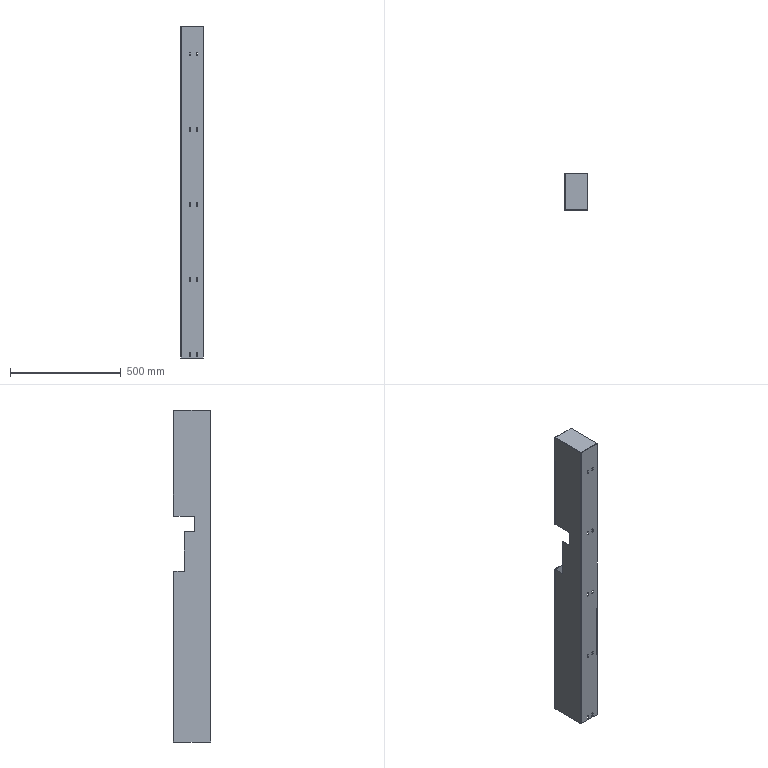Part | SolidWorks | features BaseBody 1 | 1 solid | 74 faces | box 103.5 x 169 x 1502 mm | volume 742296 mm3 | plane 46 | cylinder 28 | commonest cylinder face diameters 7 x20 1.473 x4 4.473 x4